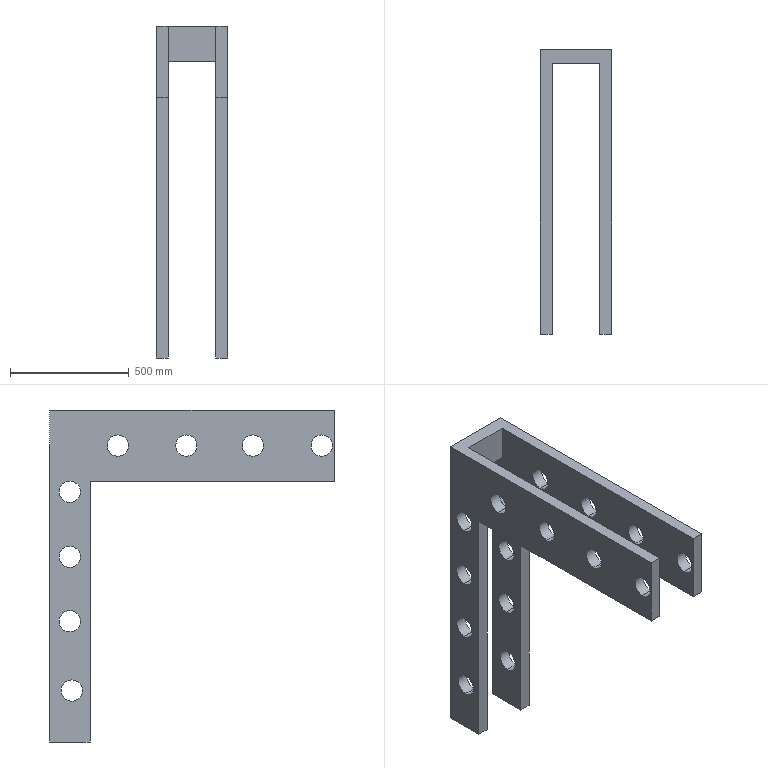Part | SolidWorks | features ICE 6, Cut 3, Extrusion 1 | 1 solid | 48 faces | box 300 x 1200 x 1400 mm | volume 51410620 mm3 | cylinder 32 | plane 16 | commonest cylinder face diameters 90 x32